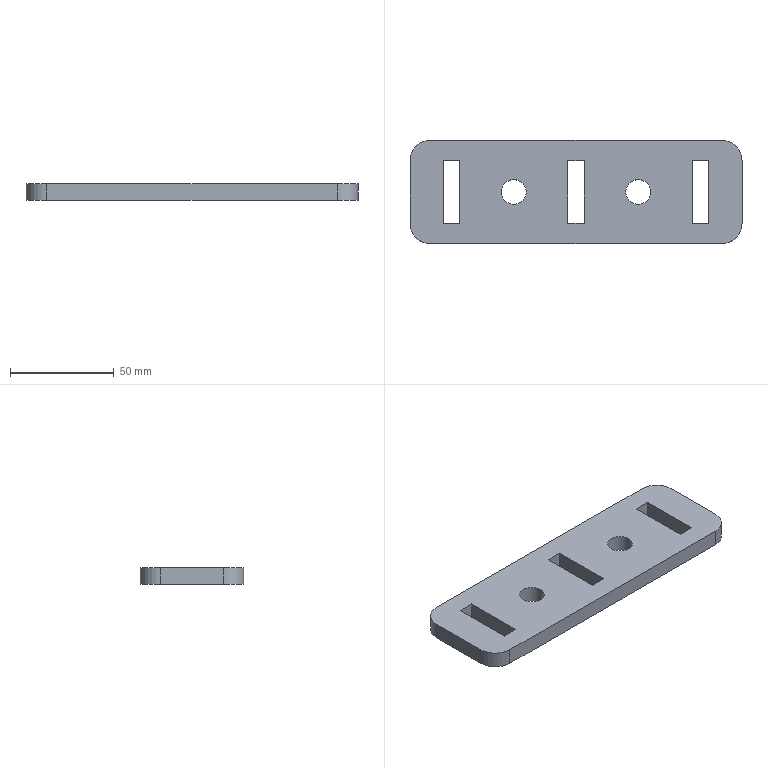Part | SolidWorks | features Fillet 1, FlatPattern 1, SMBaseFlange 1, SheetMetal 1 | 1 solid | 26 faces | box 160 x 50 x 8 mm | volume 55744 mm3 | plane 18 | cylinder 8 | commonest cylinder face diameters 12 x4 20 x4
STEP:
#1=CARTESIAN_POINT('',(-32.,480.004,8.));
#2=VERTEX_POINT('',#1);
#3=CARTESIAN_POINT('',(-20.,480.004,8.));
#4=VERTEX_POINT('',#3);
#5=CARTESIAN_POINT('',(-26.,480.004,8.));
#6=DIRECTION('',(0.,0.,1.));
#7=DIRECTION('',(1.,0.,0.));
#8=AXIS2_PLACEMENT_3D('',#5,#6,#7);
#9=CIRCLE('',#8,6.);
#10=EDGE_CURVE('',#2,#4,#9,.T.);
#11=ORIENTED_EDGE('',*,*,#10,.T.);
#12=CARTESIAN_POINT('',(-20.,480.004,0.));
#13=VERTEX_POINT('',#12);
#14=CARTESIAN_POINT('',(-20.,480.004,8.));
#15=DIRECTION('',(0.,0.,-1.));
#16=VECTOR('',#15,1000.);
#17=LINE('',#14,#16);
#18=EDGE_CURVE('',#4,#13,#17,.T.);
#19=ORIENTED_EDGE('',*,*,#18,.T.);
#20=CARTESIAN_POINT('',(-32.,480.004,0.));
#21=VERTEX_POINT('',#20);
#22=CARTESIAN_POINT('',(-26.,480.004,0.));
#23=DIRECTION('',(0.,0.,1.));
#24=DIRECTION('',(1.,0.,0.));
#25=AXIS2_PLACEMENT_3D('',#22,#23,#24);
#26=CIRCLE('',#25,6.);
#27=EDGE_CURVE('',#21,#13,#26,.T.);
#28=ORIENTED_EDGE('',*,*,#27,.F.);
#29=CARTESIAN_POINT('',(-32.,480.004,8.));
#30=DIRECTION('',(0.,0.,-1.));
#31=VECTOR('',#30,1000.);
#32=LINE('',#29,#31);
#33=EDGE_CURVE('',#2,#21,#32,.T.);
#34=ORIENTED_EDGE('',*,*,#33,.F.);
#35=EDGE_LOOP('',(#11,#19,#28,#34));
#36=FACE_OUTER_BOUND('',#35,.T.);
#37=CARTESIAN_POINT('',(-26.,480.004,8.));
#38=DIRECTION('',(0.,0.,-1.));
#39=DIRECTION('',(-1.,0.,0.));
#40=AXIS2_PLACEMENT_3D('',#37,#38,#39);
#41=CYLINDRICAL_SURFACE('',#40,6.);
#42=ADVANCED_FACE('',(#36),#41,.F.);
#43=CARTESIAN_POINT('',(28.,480.004,8.));
#44=VERTEX_POINT('',#43);
#45=CARTESIAN_POINT('',(40.,480.004,8.));
#46=VERTEX_POINT('',#45);
#47=CARTESIAN_POINT('',(34.,480.004,8.));
#48=DIRECTION('',(0.,0.,1.));
#49=DIRECTION('',(1.,0.,0.));
#50=AXIS2_PLACEMENT_3D('',#47,#48,#49);
#51=CIRCLE('',#50,6.);
#52=EDGE_CURVE('',#44,#46,#51,.T.);
#53=ORIENTED_EDGE('',*,*,#52,.T.);
#54=CARTESIAN_POINT('',(40.,480.004,0.));
#55=VERTEX_POINT('',#54);
#56=CARTESIAN_POINT('',(40.,480.004,8.));
#57=DIRECTION('',(0.,0.,-1.));
#58=VECTOR('',#57,1000.);
#59=LINE('',#56,#58);
#60=EDGE_CURVE('',#46,#55,#59,.T.);
#61=ORIENTED_EDGE('',*,*,#60,.T.);
#62=CARTESIAN_POINT('',(28.,480.004,0.));
#63=VERTEX_POINT('',#62);
#64=CARTESIAN_POINT('',(34.,480.004,0.));
#65=DIRECTION('',(0.,0.,1.));
#66=DIRECTION('',(1.,0.,0.));
#67=AXIS2_PLACEMENT_3D('',#64,#65,#66);
#68=CIRCLE('',#67,6.);
#69=EDGE_CURVE('',#63,#55,#68,.T.);
#70=ORIENTED_EDGE('',*,*,#69,.F.);
#71=CARTESIAN_POINT('',(28.,480.004,8.));
#72=DIRECTION('',(0.,0.,-1.));
#73=VECTOR('',#72,1000.);
#74=LINE('',#71,#73);
#75=EDGE_CURVE('',#44,#63,#74,.T.);
#76=ORIENTED_EDGE('',*,*,#75,.F.);
#77=EDGE_LOOP('',(#53,#61,#70,#76));
#78=FACE_OUTER_BOUND('',#77,.T.);
#79=CARTESIAN_POINT('',(34.,480.004,8.));
#80=DIRECTION('',(0.,0.,-1.));
#81=DIRECTION('',(-1.,0.,0.));
#82=AXIS2_PLACEMENT_3D('',#79,#80,#81);
#83=CYLINDRICAL_SURFACE('',#82,6.);
#84=ADVANCED_FACE('',(#78),#83,.F.);
#85=CARTESIAN_POINT('',(8.,465.004,8.));
#86=VERTEX_POINT('',#85);
#87=CARTESIAN_POINT('',(8.,495.004,8.));
#88=VERTEX_POINT('',#87);
#89=CARTESIAN_POINT('',(8.,495.004,8.));
#90=DIRECTION('',(0.,1.,0.));
#91=VECTOR('',#90,1000.);
#92=LINE('',#89,#91);
#93=EDGE_CURVE('',#86,#88,#92,.T.);
#94=ORIENTED_EDGE('',*,*,#93,.F.);
#95=CARTESIAN_POINT('',(0.,465.004,8.));
#96=VERTEX_POINT('',#95);
#97=CARTESIAN_POINT('',(8.,465.004,8.));
#98=DIRECTION('',(1.,0.,0.));
#99=VECTOR('',#98,1000.);
#100=LINE('',#97,#99);
#101=EDGE_CURVE('',#96,#86,#100,.T.);
#102=ORIENTED_EDGE('',*,*,#101,.F.);
#103=CARTESIAN_POINT('',(0.,495.004,8.));
#104=VERTEX_POINT('',#103);
#105=CARTESIAN_POINT('',(0.,495.004,8.));
#106=DIRECTION('',(0.,-1.,0.));
#107=VECTOR('',#106,1000.);
#108=LINE('',#105,#107);
#109=EDGE_CURVE('',#104,#96,#108,.T.);
#110=ORIENTED_EDGE('',*,*,#109,.F.);
#111=CARTESIAN_POINT('',(8.,495.004,8.));
#112=DIRECTION('',(-1.,0.,0.));
#113=VECTOR('',#112,1000.);
#114=LINE('',#111,#113);
#115=EDGE_CURVE('',#88,#104,#114,.T.);
#116=ORIENTED_EDGE('',*,*,#115,.F.);
#117=EDGE_LOOP('',(#94,#102,#110,#116));
#118=FACE_BOUND('',#117,.T.);
#119=CARTESIAN_POINT('',(84.,465.004,8.));
#120=VERTEX_POINT('',#119);
#121=CARTESIAN_POINT('',(84.,495.004,8.));
#122=VERTEX_POINT('',#121);
#123=CARTESIAN_POINT('',(84.,505.004,8.));
#124=DIRECTION('',(0.,1.,0.));
#125=VECTOR('',#124,1000.);
#126=LINE('',#123,#125);
#127=EDGE_CURVE('',#120,#122,#126,.T.);
#128=ORIENTED_EDGE('',*,*,#127,.T.);
#129=CARTESIAN_POINT('',(74.,505.004,8.));
#130=VERTEX_POINT('',#129);
#131=CARTESIAN_POINT('',(74.,495.004,8.));
#132=DIRECTION('',(0.,0.,1.));
#133=DIRECTION('',(-1.,0.,0.));
#134=AXIS2_PLACEMENT_3D('',#131,#132,#133);
#135=CIRCLE('',#134,10.);
#136=EDGE_CURVE('',#122,#130,#135,.T.);
#137=ORIENTED_EDGE('',*,*,#136,.T.);
#138=CARTESIAN_POINT('',(-66.,505.004,8.));
#139=VERTEX_POINT('',#138);
#140=CARTESIAN_POINT('',(84.,505.004,8.));
#141=DIRECTION('',(-1.,0.,0.));
#142=VECTOR('',#141,1000.);
#143=LINE('',#140,#142);
#144=EDGE_CURVE('',#130,#139,#143,.T.);
#145=ORIENTED_EDGE('',*,*,#144,.T.);
#146=CARTESIAN_POINT('',(-76.,495.004,8.));
#147=VERTEX_POINT('',#146);
#148=CARTESIAN_POINT('',(-66.,495.004,8.));
#149=DIRECTION('',(0.,0.,1.));
#150=DIRECTION('',(-1.,0.,0.));
#151=AXIS2_PLACEMENT_3D('',#148,#149,#150);
#152=CIRCLE('',#151,10.);
#153=EDGE_CURVE('',#139,#147,#152,.T.);
#154=ORIENTED_EDGE('',*,*,#153,.T.);
#155=CARTESIAN_POINT('',(-76.,465.004,8.));
#156=VERTEX_POINT('',#155);
#157=CARTESIAN_POINT('',(-76.,505.004,8.));
#158=DIRECTION('',(0.,-1.,0.));
#159=VECTOR('',#158,1000.);
#160=LINE('',#157,#159);
#161=EDGE_CURVE('',#147,#156,#160,.T.);
#162=ORIENTED_EDGE('',*,*,#161,.T.);
#163=CARTESIAN_POINT('',(-66.,455.004,8.));
#164=VERTEX_POINT('',#163);
#165=CARTESIAN_POINT('',(-66.,465.004,8.));
#166=DIRECTION('',(0.,0.,1.));
#167=DIRECTION('',(-1.,0.,0.));
#168=AXIS2_PLACEMENT_3D('',#165,#166,#167);
#169=CIRCLE('',#168,10.);
#170=EDGE_CURVE('',#156,#164,#169,.T.);
#171=ORIENTED_EDGE('',*,*,#170,.T.);
#172=CARTESIAN_POINT('',(74.,455.004,8.));
#173=VERTEX_POINT('',#172);
#174=CARTESIAN_POINT('',(84.,455.004,8.));
#175=DIRECTION('',(1.,0.,0.));
#176=VECTOR('',#175,1000.);
#177=LINE('',#174,#176);
#178=EDGE_CURVE('',#164,#173,#177,.T.);
#179=ORIENTED_EDGE('',*,*,#178,.T.);
#180=CARTESIAN_POINT('',(74.,465.004,8.));
#181=DIRECTION('',(0.,0.,1.));
#182=DIRECTION('',(-1.,0.,0.));
#183=AXIS2_PLACEMENT_3D('',#180,#181,#182);
#184=CIRCLE('',#183,10.);
#185=EDGE_CURVE('',#173,#120,#184,.T.);
#186=ORIENTED_EDGE('',*,*,#185,.T.);
#187=EDGE_LOOP('',(#128,#137,#145,#154,#162,#171,#179,#186));
#188=FACE_OUTER_BOUND('',#187,.T.);
#189=CARTESIAN_POINT('',(68.,465.004,8.));
#190=VERTEX_POINT('',#189);
#191=CARTESIAN_POINT('',(68.,495.004,8.));
#192=VERTEX_POINT('',#191);
#193=CARTESIAN_POINT('',(68.,495.004,8.));
#194=DIRECTION('',(0.,1.,0.));
#195=VECTOR('',#194,1000.);
#196=LINE('',#193,#195);
#197=EDGE_CURVE('',#190,#192,#196,.T.);
#198=ORIENTED_EDGE('',*,*,#197,.F.);
#199=CARTESIAN_POINT('',(60.,465.004,8.));
#200=VERTEX_POINT('',#199);
#201=CARTESIAN_POINT('',(68.,465.004,8.));
#202=DIRECTION('',(1.,0.,0.));
#203=VECTOR('',#202,1000.);
#204=LINE('',#201,#203);
#205=EDGE_CURVE('',#200,#190,#204,.T.);
#206=ORIENTED_EDGE('',*,*,#205,.F.);
#207=CARTESIAN_POINT('',(60.,495.004,8.));
#208=VERTEX_POINT('',#207);
#209=CARTESIAN_POINT('',(60.,495.004,8.));
#210=DIRECTION('',(0.,-1.,0.));
#211=VECTOR('',#210,1000.);
#212=LINE('',#209,#211);
#213=EDGE_CURVE('',#208,#200,#212,.T.);
#214=ORIENTED_EDGE('',*,*,#213,.F.);
#215=CARTESIAN_POINT('',(68.,495.004,8.));
#216=DIRECTION('',(-1.,0.,0.));
#217=VECTOR('',#216,1000.);
#218=LINE('',#215,#217);
#219=EDGE_CURVE('',#192,#208,#218,.T.);
#220=ORIENTED_EDGE('',*,*,#219,.F.);
#221=EDGE_LOOP('',(#198,#206,#214,#220));
#222=FACE_BOUND('',#221,.T.);
#223=CARTESIAN_POINT('',(-60.,495.004,8.));
#224=VERTEX_POINT('',#223);
#225=CARTESIAN_POINT('',(-60.,465.004,8.));
#226=VERTEX_POINT('',#225);
#227=CARTESIAN_POINT('',(-60.,465.004,8.));
#228=DIRECTION('',(0.,-1.,0.));
#229=VECTOR('',#228,1000.);
#230=LINE('',#227,#229);
#231=EDGE_CURVE('',#224,#226,#230,.T.);
#232=ORIENTED_EDGE('',*,*,#231,.F.);
#233=CARTESIAN_POINT('',(-52.,495.004,8.));
#234=VERTEX_POINT('',#233);
#235=CARTESIAN_POINT('',(-60.,495.004,8.));
#236=DIRECTION('',(-1.,0.,0.));
#237=VECTOR('',#236,1000.);
#238=LINE('',#235,#237);
#239=EDGE_CURVE('',#234,#224,#238,.T.);
#240=ORIENTED_EDGE('',*,*,#239,.F.);
#241=CARTESIAN_POINT('',(-52.,465.004,8.));
#242=VERTEX_POINT('',#241);
#243=CARTESIAN_POINT('',(-52.,465.004,8.));
#244=DIRECTION('',(0.,1.,0.));
#245=VECTOR('',#244,1000.);
#246=LINE('',#243,#245);
#247=EDGE_CURVE('',#242,#234,#246,.T.);
#248=ORIENTED_EDGE('',*,*,#247,.F.);
#249=CARTESIAN_POINT('',(-60.,465.004,8.));
#250=DIRECTION('',(1.,0.,0.));
#251=VECTOR('',#250,1000.);
#252=LINE('',#249,#251);
#253=EDGE_CURVE('',#226,#242,#252,.T.);
#254=ORIENTED_EDGE('',*,*,#253,.F.);
#255=EDGE_LOOP('',(#232,#240,#248,#254));
#256=FACE_BOUND('',#255,.T.);
#257=ORIENTED_EDGE('',*,*,#52,.F.);
#258=CARTESIAN_POINT('',(34.,480.004,8.));
#259=DIRECTION('',(0.,0.,1.));
#260=DIRECTION('',(1.,0.,0.));
#261=AXIS2_PLACEMENT_3D('',#258,#259,#260);
#262=CIRCLE('',#261,6.);
#263=EDGE_CURVE('',#46,#44,#262,.T.);
#264=ORIENTED_EDGE('',*,*,#263,.F.);
#265=EDGE_LOOP('',(#257,#264));
#266=FACE_BOUND('',#265,.T.);
#267=ORIENTED_EDGE('',*,*,#10,.F.);
#268=CARTESIAN_POINT('',(-26.,480.004,8.));
#269=DIRECTION('',(0.,0.,1.));
#270=DIRECTION('',(1.,0.,0.));
#271=AXIS2_PLACEMENT_3D('',#268,#269,#270);
#272=CIRCLE('',#271,6.);
#273=EDGE_CURVE('',#4,#2,#272,.T.);
#274=ORIENTED_EDGE('',*,*,#273,.F.);
#275=EDGE_LOOP('',(#267,#274));
#276=FACE_BOUND('',#275,.T.);
#277=CARTESIAN_POINT('',(0.,0.,8.));
#278=DIRECTION('',(0.,0.,-1.));
#279=DIRECTION('',(-1.,0.,0.));
#280=AXIS2_PLACEMENT_3D('',#277,#278,#279);
#281=PLANE('',#280);
#282=ADVANCED_FACE('',(#118,#188,#222,#256,#266,#276),#281,.F.);
#283=ORIENTED_EDGE('',*,*,#69,.T.);
#284=CARTESIAN_POINT('',(34.,480.004,0.));
#285=DIRECTION('',(0.,0.,1.));
#286=DIRECTION('',(1.,0.,0.));
#287=AXIS2_PLACEMENT_3D('',#284,#285,#286);
#288=CIRCLE('',#287,6.);
#289=EDGE_CURVE('',#55,#63,#288,.T.);
#290=ORIENTED_EDGE('',*,*,#289,.T.);
#291=EDGE_LOOP('',(#283,#290));
#292=FACE_BOUND('',#291,.T.);
#293=CARTESIAN_POINT('',(74.,505.004,0.));
#294=VERTEX_POINT('',#293);
#295=CARTESIAN_POINT('',(-66.,505.004,0.));
#296=VERTEX_POINT('',#295);
#297=CARTESIAN_POINT('',(84.,505.004,0.));
#298=DIRECTION('',(-1.,0.,0.));
#299=VECTOR('',#298,1000.);
#300=LINE('',#297,#299);
#301=EDGE_CURVE('',#294,#296,#300,.T.);
#302=ORIENTED_EDGE('',*,*,#301,.F.);
#303=CARTESIAN_POINT('',(84.,495.004,0.));
#304=VERTEX_POINT('',#303);
#305=CARTESIAN_POINT('',(74.,495.004,0.));
#306=DIRECTION('',(0.,0.,-1.));
#307=DIRECTION('',(-1.,0.,0.));
#308=AXIS2_PLACEMENT_3D('',#305,#306,#307);
#309=CIRCLE('',#308,10.);
#310=EDGE_CURVE('',#294,#304,#309,.T.);
#311=ORIENTED_EDGE('',*,*,#310,.T.);
#312=CARTESIAN_POINT('',(84.,465.004,0.));
#313=VERTEX_POINT('',#312);
#314=CARTESIAN_POINT('',(84.,505.004,0.));
#315=DIRECTION('',(0.,1.,0.));
#316=VECTOR('',#315,1000.);
#317=LINE('',#314,#316);
#318=EDGE_CURVE('',#313,#304,#317,.T.);
#319=ORIENTED_EDGE('',*,*,#318,.F.);
#320=CARTESIAN_POINT('',(74.,455.004,0.));
#321=VERTEX_POINT('',#320);
#322=CARTESIAN_POINT('',(74.,465.004,0.));
#323=DIRECTION('',(0.,0.,-1.));
#324=DIRECTION('',(-1.,0.,0.));
#325=AXIS2_PLACEMENT_3D('',#322,#323,#324);
#326=CIRCLE('',#325,10.);
#327=EDGE_CURVE('',#313,#321,#326,.T.);
#328=ORIENTED_EDGE('',*,*,#327,.T.);
#329=CARTESIAN_POINT('',(-66.,455.004,0.));
#330=VERTEX_POINT('',#329);
#331=CARTESIAN_POINT('',(84.,455.004,0.));
#332=DIRECTION('',(1.,0.,0.));
#333=VECTOR('',#332,1000.);
#334=LINE('',#331,#333);
#335=EDGE_CURVE('',#330,#321,#334,.T.);
#336=ORIENTED_EDGE('',*,*,#335,.F.);
#337=CARTESIAN_POINT('',(-76.,465.004,0.));
#338=VERTEX_POINT('',#337);
#339=CARTESIAN_POINT('',(-66.,465.004,0.));
#340=DIRECTION('',(0.,0.,-1.));
#341=DIRECTION('',(-1.,0.,0.));
#342=AXIS2_PLACEMENT_3D('',#339,#340,#341);
#343=CIRCLE('',#342,10.);
#344=EDGE_CURVE('',#330,#338,#343,.T.);
#345=ORIENTED_EDGE('',*,*,#344,.T.);
#346=CARTESIAN_POINT('',(-76.,495.004,0.));
#347=VERTEX_POINT('',#346);
#348=CARTESIAN_POINT('',(-76.,505.004,0.));
#349=DIRECTION('',(0.,-1.,0.));
#350=VECTOR('',#349,1000.);
#351=LINE('',#348,#350);
#352=EDGE_CURVE('',#347,#338,#351,.T.);
#353=ORIENTED_EDGE('',*,*,#352,.F.);
#354=CARTESIAN_POINT('',(-66.,495.004,0.));
#355=DIRECTION('',(0.,0.,-1.));
#356=DIRECTION('',(-1.,0.,0.));
#357=AXIS2_PLACEMENT_3D('',#354,#355,#356);
#358=CIRCLE('',#357,10.);
#359=EDGE_CURVE('',#347,#296,#358,.T.);
#360=ORIENTED_EDGE('',*,*,#359,.T.);
#361=EDGE_LOOP('',(#302,#311,#319,#328,#336,#345,#353,#360));
#362=FACE_OUTER_BOUND('',#361,.T.);
#363=CARTESIAN_POINT('',(60.,465.004,0.));
#364=VERTEX_POINT('',#363);
#365=CARTESIAN_POINT('',(68.,465.004,0.));
#366=VERTEX_POINT('',#365);
#367=CARTESIAN_POINT('',(68.,465.004,0.));
#368=DIRECTION('',(1.,0.,0.));
#369=VECTOR('',#368,1000.);
#370=LINE('',#367,#369);
#371=EDGE_CURVE('',#364,#366,#370,.T.);
#372=ORIENTED_EDGE('',*,*,#371,.T.);
#373=CARTESIAN_POINT('',(68.,495.004,0.));
#374=VERTEX_POINT('',#373);
#375=CARTESIAN_POINT('',(68.,495.004,0.));
#376=DIRECTION('',(0.,1.,0.));
#377=VECTOR('',#376,1000.);
#378=LINE('',#375,#377);
#379=EDGE_CURVE('',#366,#374,#378,.T.);
#380=ORIENTED_EDGE('',*,*,#379,.T.);
#381=CARTESIAN_POINT('',(60.,495.004,0.));
#382=VERTEX_POINT('',#381);
#383=CARTESIAN_POINT('',(68.,495.004,0.));
#384=DIRECTION('',(-1.,0.,0.));
#385=VECTOR('',#384,1000.);
#386=LINE('',#383,#385);
#387=EDGE_CURVE('',#374,#382,#386,.T.);
#388=ORIENTED_EDGE('',*,*,#387,.T.);
#389=CARTESIAN_POINT('',(60.,495.004,0.));
#390=DIRECTION('',(0.,-1.,0.));
#391=VECTOR('',#390,1000.);
#392=LINE('',#389,#391);
#393=EDGE_CURVE('',#382,#364,#392,.T.);
#394=ORIENTED_EDGE('',*,*,#393,.T.);
#395=EDGE_LOOP('',(#372,#380,#388,#394));
#396=FACE_BOUND('',#395,.T.);
#397=CARTESIAN_POINT('',(0.,465.004,0.));
#398=VERTEX_POINT('',#397);
#399=CARTESIAN_POINT('',(8.,465.004,0.));
#400=VERTEX_POINT('',#399);
#401=CARTESIAN_POINT('',(8.,465.004,0.));
#402=DIRECTION('',(1.,0.,0.));
#403=VECTOR('',#402,1000.);
#404=LINE('',#401,#403);
#405=EDGE_CURVE('',#398,#400,#404,.T.);
#406=ORIENTED_EDGE('',*,*,#405,.T.);
#407=CARTESIAN_POINT('',(8.,495.004,0.));
#408=VERTEX_POINT('',#407);
#409=CARTESIAN_POINT('',(8.,495.004,0.));
#410=DIRECTION('',(0.,1.,0.));
#411=VECTOR('',#410,1000.);
#412=LINE('',#409,#411);
#413=EDGE_CURVE('',#400,#408,#412,.T.);
#414=ORIENTED_EDGE('',*,*,#413,.T.);
#415=CARTESIAN_POINT('',(0.,495.004,0.));
#416=VERTEX_POINT('',#415);
#417=CARTESIAN_POINT('',(8.,495.004,0.));
#418=DIRECTION('',(-1.,0.,0.));
#419=VECTOR('',#418,1000.);
#420=LINE('',#417,#419);
#421=EDGE_CURVE('',#408,#416,#420,.T.);
#422=ORIENTED_EDGE('',*,*,#421,.T.);
#423=CARTESIAN_POINT('',(0.,495.004,0.));
#424=DIRECTION('',(0.,-1.,0.));
#425=VECTOR('',#424,1000.);
#426=LINE('',#423,#425);
#427=EDGE_CURVE('',#416,#398,#426,.T.);
#428=ORIENTED_EDGE('',*,*,#427,.T.);
#429=EDGE_LOOP('',(#406,#414,#422,#428));
#430=FACE_BOUND('',#429,.T.);
#431=CARTESIAN_POINT('',(-52.,495.004,0.));
#432=VERTEX_POINT('',#431);
#433=CARTESIAN_POINT('',(-60.,495.004,0.));
#434=VERTEX_POINT('',#433);
#435=CARTESIAN_POINT('',(-60.,495.004,0.));
#436=DIRECTION('',(-1.,0.,0.));
#437=VECTOR('',#436,1000.);
#438=LINE('',#435,#437);
#439=EDGE_CURVE('',#432,#434,#438,.T.);
#440=ORIENTED_EDGE('',*,*,#439,.T.);
#441=CARTESIAN_POINT('',(-60.,465.004,0.));
#442=VERTEX_POINT('',#441);
#443=CARTESIAN_POINT('',(-60.,465.004,0.));
#444=DIRECTION('',(0.,-1.,0.));
#445=VECTOR('',#444,1000.);
#446=LINE('',#443,#445);
#447=EDGE_CURVE('',#434,#442,#446,.T.);
#448=ORIENTED_EDGE('',*,*,#447,.T.);
#449=CARTESIAN_POINT('',(-52.,465.004,0.));
#450=VERTEX_POINT('',#449);
#451=CARTESIAN_POINT('',(-60.,465.004,0.));
#452=DIRECTION('',(1.,0.,0.));
#453=VECTOR('',#452,1000.);
#454=LINE('',#451,#453);
#455=EDGE_CURVE('',#442,#450,#454,.T.);
#456=ORIENTED_EDGE('',*,*,#455,.T.);
#457=CARTESIAN_POINT('',(-52.,465.004,0.));
#458=DIRECTION('',(0.,1.,0.));
#459=VECTOR('',#458,1000.);
#460=LINE('',#457,#459);
#461=EDGE_CURVE('',#450,#432,#460,.T.);
#462=ORIENTED_EDGE('',*,*,#461,.T.);
#463=EDGE_LOOP('',(#440,#448,#456,#462));
#464=FACE_BOUND('',#463,.T.);
#465=ORIENTED_EDGE('',*,*,#27,.T.);
#466=CARTESIAN_POINT('',(-26.,480.004,0.));
#467=DIRECTION('',(0.,0.,1.));
#468=DIRECTION('',(1.,0.,0.));
#469=AXIS2_PLACEMENT_3D('',#466,#467,#468);
#470=CIRCLE('',#469,6.);
#471=EDGE_CURVE('',#13,#21,#470,.T.);
#472=ORIENTED_EDGE('',*,*,#471,.T.);
#473=EDGE_LOOP('',(#465,#472));
#474=FACE_BOUND('',#473,.T.);
#475=CARTESIAN_POINT('',(0.,0.,0.));
#476=DIRECTION('',(0.,0.,-1.));
#477=DIRECTION('',(-1.,0.,0.));
#478=AXIS2_PLACEMENT_3D('',#475,#476,#477);
#479=PLANE('',#478);
#480=ADVANCED_FACE('',(#292,#362,#396,#430,#464,#474),#479,.T.);
#481=ORIENTED_EDGE('',*,*,#318,.T.);
#482=CARTESIAN_POINT('',(84.,495.004,8.));
#483=DIRECTION('',(0.,0.,1.));
#484=VECTOR('',#483,1000.);
#485=LINE('',#482,#484);
#486=EDGE_CURVE('',#304,#122,#485,.T.);
#487=ORIENTED_EDGE('',*,*,#486,.T.);
#488=ORIENTED_EDGE('',*,*,#127,.F.);
#489=CARTESIAN_POINT('',(84.,465.004,8.));
#490=DIRECTION('',(0.,0.,-1.));
#491=VECTOR('',#490,1000.);
#492=LINE('',#489,#491);
#493=EDGE_CURVE('',#120,#313,#492,.T.);
#494=ORIENTED_EDGE('',*,*,#493,.T.);
#495=EDGE_LOOP('',(#481,#487,#488,#494));
#496=FACE_OUTER_BOUND('',#495,.T.);
#497=CARTESIAN_POINT('',(84.,505.004,8.));
#498=DIRECTION('',(-1.,0.,0.));
#499=DIRECTION('',(0.,0.,1.));
#500=AXIS2_PLACEMENT_3D('',#497,#498,#499);
#501=PLANE('',#500);
#502=ADVANCED_FACE('',(#496),#501,.F.);
#503=ORIENTED_EDGE('',*,*,#144,.F.);
#504=CARTESIAN_POINT('',(74.,505.004,8.));
#505=DIRECTION('',(0.,0.,-1.));
#506=VECTOR('',#505,1000.);
#507=LINE('',#504,#506);
#508=EDGE_CURVE('',#130,#294,#507,.T.);
#509=ORIENTED_EDGE('',*,*,#508,.T.);
#510=ORIENTED_EDGE('',*,*,#301,.T.);
#511=CARTESIAN_POINT('',(-66.,505.004,8.));
#512=DIRECTION('',(0.,0.,1.));
#513=VECTOR('',#512,1000.);
#514=LINE('',#511,#513);
#515=EDGE_CURVE('',#296,#139,#514,.T.);
#516=ORIENTED_EDGE('',*,*,#515,.T.);
#517=EDGE_LOOP('',(#503,#509,#510,#516));
#518=FACE_OUTER_BOUND('',#517,.T.);
#519=CARTESIAN_POINT('',(84.,505.004,8.));
#520=DIRECTION('',(0.,-1.,0.));
#521=DIRECTION('',(0.,0.,-1.));
#522=AXIS2_PLACEMENT_3D('',#519,#520,#521);
#523=PLANE('',#522);
#524=ADVANCED_FACE('',(#518),#523,.F.);
#525=ORIENTED_EDGE('',*,*,#161,.F.);
#526=CARTESIAN_POINT('',(-76.,495.004,8.));
#527=DIRECTION('',(0.,0.,-1.));
#528=VECTOR('',#527,1000.);
#529=LINE('',#526,#528);
#530=EDGE_CURVE('',#147,#347,#529,.T.);
#531=ORIENTED_EDGE('',*,*,#530,.T.);
#532=ORIENTED_EDGE('',*,*,#352,.T.);
#533=CARTESIAN_POINT('',(-76.,465.004,8.));
#534=DIRECTION('',(0.,0.,1.));
#535=VECTOR('',#534,1000.);
#536=LINE('',#533,#535);
#537=EDGE_CURVE('',#338,#156,#536,.T.);
#538=ORIENTED_EDGE('',*,*,#537,.T.);
#539=EDGE_LOOP('',(#525,#531,#532,#538));
#540=FACE_OUTER_BOUND('',#539,.T.);
#541=CARTESIAN_POINT('',(-76.,505.004,8.));
#542=DIRECTION('',(1.,0.,0.));
#543=DIRECTION('',(0.,0.,-1.));
#544=AXIS2_PLACEMENT_3D('',#541,#542,#543);
#545=PLANE('',#544);
#546=ADVANCED_FACE('',(#540),#545,.F.);
#547=ORIENTED_EDGE('',*,*,#335,.T.);
#548=CARTESIAN_POINT('',(74.,455.004,8.));
#549=DIRECTION('',(0.,0.,1.));
#550=VECTOR('',#549,1000.);
#551=LINE('',#548,#550);
#552=EDGE_CURVE('',#321,#173,#551,.T.);
#553=ORIENTED_EDGE('',*,*,#552,.T.);
#554=ORIENTED_EDGE('',*,*,#178,.F.);
#555=CARTESIAN_POINT('',(-66.,455.004,8.));
#556=DIRECTION('',(0.,0.,-1.));
#557=VECTOR('',#556,1000.);
#558=LINE('',#555,#557);
#559=EDGE_CURVE('',#164,#330,#558,.T.);
#560=ORIENTED_EDGE('',*,*,#559,.T.);
#561=EDGE_LOOP('',(#547,#553,#554,#560));
#562=FACE_OUTER_BOUND('',#561,.T.);
#563=CARTESIAN_POINT('',(84.,455.004,8.));
#564=DIRECTION('',(0.,1.,0.));
#565=DIRECTION('',(0.,0.,1.));
#566=AXIS2_PLACEMENT_3D('',#563,#564,#565);
#567=PLANE('',#566);
#568=ADVANCED_FACE('',(#562),#567,.F.);
#569=ORIENTED_EDGE('',*,*,#379,.F.);
#570=CARTESIAN_POINT('',(68.,465.004,8.));
#571=DIRECTION('',(0.,0.,-1.));
#572=VECTOR('',#571,1000.);
#573=LINE('',#570,#572);
#574=EDGE_CURVE('',#190,#366,#573,.T.);
#575=ORIENTED_EDGE('',*,*,#574,.F.);
#576=ORIENTED_EDGE('',*,*,#197,.T.);
#577=CARTESIAN_POINT('',(68.,495.004,8.));
#578=DIRECTION('',(0.,0.,-1.));
#579=VECTOR('',#578,1000.);
#580=LINE('',#577,#579);
#581=EDGE_CURVE('',#192,#374,#580,.T.);
#582=ORIENTED_EDGE('',*,*,#581,.T.);
#583=EDGE_LOOP('',(#569,#575,#576,#582));
#584=FACE_OUTER_BOUND('',#583,.T.);
#585=CARTESIAN_POINT('',(68.,495.004,8.));
#586=DIRECTION('',(-1.,0.,0.));
#587=DIRECTION('',(0.,0.,1.));
#588=AXIS2_PLACEMENT_3D('',#585,#586,#587);
#589=PLANE('',#588);
#590=ADVANCED_FACE('',(#584),#589,.T.);
#591=ORIENTED_EDGE('',*,*,#387,.F.);
#592=ORIENTED_EDGE('',*,*,#581,.F.);
#593=ORIENTED_EDGE('',*,*,#219,.T.);
#594=CARTESIAN_POINT('',(60.,495.004,8.));
#595=DIRECTION('',(0.,0.,-1.));
#596=VECTOR('',#595,1000.);
#597=LINE('',#594,#596);
#598=EDGE_CURVE('',#208,#382,#597,.T.);
#599=ORIENTED_EDGE('',*,*,#598,.T.);
#600=EDGE_LOOP('',(#591,#592,#593,#599));
#601=FACE_OUTER_BOUND('',#600,.T.);
#602=CARTESIAN_POINT('',(68.,495.004,8.));
#603=DIRECTION('',(0.,-1.,0.));
#604=DIRECTION('',(0.,0.,-1.));
#605=AXIS2_PLACEMENT_3D('',#602,#603,#604);
#606=PLANE('',#605);
#607=ADVANCED_FACE('',(#601),#606,.T.);
#608=ORIENTED_EDGE('',*,*,#393,.F.);
#609=ORIENTED_EDGE('',*,*,#598,.F.);
#610=ORIENTED_EDGE('',*,*,#213,.T.);
#611=CARTESIAN_POINT('',(60.,465.004,8.));
#612=DIRECTION('',(0.,0.,-1.));
#613=VECTOR('',#612,1000.);
#614=LINE('',#611,#613);
#615=EDGE_CURVE('',#200,#364,#614,.T.);
#616=ORIENTED_EDGE('',*,*,#615,.T.);
#617=EDGE_LOOP('',(#608,#609,#610,#616));
#618=FACE_OUTER_BOUND('',#617,.T.);
#619=CARTESIAN_POINT('',(60.,495.004,8.));
#620=DIRECTION('',(1.,0.,0.));
#621=DIRECTION('',(0.,0.,-1.));
#622=AXIS2_PLACEMENT_3D('',#619,#620,#621);
#623=PLANE('',#622);
#624=ADVANCED_FACE('',(#618),#623,.T.);
#625=ORIENTED_EDGE('',*,*,#371,.F.);
#626=ORIENTED_EDGE('',*,*,#615,.F.);
#627=ORIENTED_EDGE('',*,*,#205,.T.);
#628=ORIENTED_EDGE('',*,*,#574,.T.);
#629=EDGE_LOOP('',(#625,#626,#627,#628));
#630=FACE_OUTER_BOUND('',#629,.T.);
#631=CARTESIAN_POINT('',(68.,465.004,8.));
#632=DIRECTION('',(0.,1.,0.));
#633=DIRECTION('',(0.,0.,1.));
#634=AXIS2_PLACEMENT_3D('',#631,#632,#633);
#635=PLANE('',#634);
#636=ADVANCED_FACE('',(#630),#635,.T.);
#637=ORIENTED_EDGE('',*,*,#413,.F.);
#638=CARTESIAN_POINT('',(8.,465.004,8.));
#639=DIRECTION('',(0.,0.,-1.));
#640=VECTOR('',#639,1000.);
#641=LINE('',#638,#640);
#642=EDGE_CURVE('',#86,#400,#641,.T.);
#643=ORIENTED_EDGE('',*,*,#642,.F.);
#644=ORIENTED_EDGE('',*,*,#93,.T.);
#645=CARTESIAN_POINT('',(8.,495.004,8.));
#646=DIRECTION('',(0.,0.,-1.));
#647=VECTOR('',#646,1000.);
#648=LINE('',#645,#647);
#649=EDGE_CURVE('',#88,#408,#648,.T.);
#650=ORIENTED_EDGE('',*,*,#649,.T.);
#651=EDGE_LOOP('',(#637,#643,#644,#650));
#652=FACE_OUTER_BOUND('',#651,.T.);
#653=CARTESIAN_POINT('',(8.,495.004,8.));
#654=DIRECTION('',(-1.,0.,0.));
#655=DIRECTION('',(0.,0.,1.));
#656=AXIS2_PLACEMENT_3D('',#653,#654,#655);
#657=PLANE('',#656);
#658=ADVANCED_FACE('',(#652),#657,.T.);
#659=ORIENTED_EDGE('',*,*,#421,.F.);
#660=ORIENTED_EDGE('',*,*,#649,.F.);
#661=ORIENTED_EDGE('',*,*,#115,.T.);
#662=CARTESIAN_POINT('',(0.,495.004,8.));
#663=DIRECTION('',(0.,0.,-1.));
#664=VECTOR('',#663,1000.);
#665=LINE('',#662,#664);
#666=EDGE_CURVE('',#104,#416,#665,.T.);
#667=ORIENTED_EDGE('',*,*,#666,.T.);
#668=EDGE_LOOP('',(#659,#660,#661,#667));
#669=FACE_OUTER_BOUND('',#668,.T.);
#670=CARTESIAN_POINT('',(8.,495.004,8.));
#671=DIRECTION('',(0.,-1.,0.));
#672=DIRECTION('',(0.,0.,-1.));
#673=AXIS2_PLACEMENT_3D('',#670,#671,#672);
#674=PLANE('',#673);
#675=ADVANCED_FACE('',(#669),#674,.T.);
#676=ORIENTED_EDGE('',*,*,#427,.F.);
#677=ORIENTED_EDGE('',*,*,#666,.F.);
#678=ORIENTED_EDGE('',*,*,#109,.T.);
#679=CARTESIAN_POINT('',(0.,465.004,8.));
#680=DIRECTION('',(0.,0.,-1.));
#681=VECTOR('',#680,1000.);
#682=LINE('',#679,#681);
#683=EDGE_CURVE('',#96,#398,#682,.T.);
#684=ORIENTED_EDGE('',*,*,#683,.T.);
#685=EDGE_LOOP('',(#676,#677,#678,#684));
#686=FACE_OUTER_BOUND('',#685,.T.);
#687=CARTESIAN_POINT('',(0.,495.004,8.));
#688=DIRECTION('',(1.,0.,0.));
#689=DIRECTION('',(0.,0.,-1.));
#690=AXIS2_PLACEMENT_3D('',#687,#688,#689);
#691=PLANE('',#690);
#692=ADVANCED_FACE('',(#686),#691,.T.);
#693=ORIENTED_EDGE('',*,*,#405,.F.);
#694=ORIENTED_EDGE('',*,*,#683,.F.);
#695=ORIENTED_EDGE('',*,*,#101,.T.);
#696=ORIENTED_EDGE('',*,*,#642,.T.);
#697=EDGE_LOOP('',(#693,#694,#695,#696));
#698=FACE_OUTER_BOUND('',#697,.T.);
#699=CARTESIAN_POINT('',(8.,465.004,8.));
#700=DIRECTION('',(0.,1.,0.));
#701=DIRECTION('',(0.,0.,1.));
#702=AXIS2_PLACEMENT_3D('',#699,#700,#701);
#703=PLANE('',#702);
#704=ADVANCED_FACE('',(#698),#703,.T.);
#705=ORIENTED_EDGE('',*,*,#447,.F.);
#706=CARTESIAN_POINT('',(-60.,495.004,8.));
#707=DIRECTION('',(0.,0.,-1.));
#708=VECTOR('',#707,1000.);
#709=LINE('',#706,#708);
#710=EDGE_CURVE('',#224,#434,#709,.T.);
#711=ORIENTED_EDGE('',*,*,#710,.F.);
#712=ORIENTED_EDGE('',*,*,#231,.T.);
#713=CARTESIAN_POINT('',(-60.,465.004,8.));
#714=DIRECTION('',(0.,0.,-1.));
#715=VECTOR('',#714,1000.);
#716=LINE('',#713,#715);
#717=EDGE_CURVE('',#226,#442,#716,.T.);
#718=ORIENTED_EDGE('',*,*,#717,.T.);
#719=EDGE_LOOP('',(#705,#711,#712,#718));
#720=FACE_OUTER_BOUND('',#719,.T.);
#721=CARTESIAN_POINT('',(-60.,465.004,8.));
#722=DIRECTION('',(1.,0.,0.));
#723=DIRECTION('',(0.,0.,-1.));
#724=AXIS2_PLACEMENT_3D('',#721,#722,#723);
#725=PLANE('',#724);
#726=ADVANCED_FACE('',(#720),#725,.T.);
#727=ORIENTED_EDGE('',*,*,#455,.F.);
#728=ORIENTED_EDGE('',*,*,#717,.F.);
#729=ORIENTED_EDGE('',*,*,#253,.T.);
#730=CARTESIAN_POINT('',(-52.,465.004,8.));
#731=DIRECTION('',(0.,0.,-1.));
#732=VECTOR('',#731,1000.);
#733=LINE('',#730,#732);
#734=EDGE_CURVE('',#242,#450,#733,.T.);
#735=ORIENTED_EDGE('',*,*,#734,.T.);
#736=EDGE_LOOP('',(#727,#728,#729,#735));
#737=FACE_OUTER_BOUND('',#736,.T.);
#738=CARTESIAN_POINT('',(-60.,465.004,8.));
#739=DIRECTION('',(0.,1.,0.));
#740=DIRECTION('',(0.,0.,1.));
#741=AXIS2_PLACEMENT_3D('',#738,#739,#740);
#742=PLANE('',#741);
#743=ADVANCED_FACE('',(#737),#742,.T.);
#744=ORIENTED_EDGE('',*,*,#461,.F.);
#745=ORIENTED_EDGE('',*,*,#734,.F.);
#746=ORIENTED_EDGE('',*,*,#247,.T.);
#747=CARTESIAN_POINT('',(-52.,495.004,8.));
#748=DIRECTION('',(0.,0.,-1.));
#749=VECTOR('',#748,1000.);
#750=LINE('',#747,#749);
#751=EDGE_CURVE('',#234,#432,#750,.T.);
#752=ORIENTED_EDGE('',*,*,#751,.T.);
#753=EDGE_LOOP('',(#744,#745,#746,#752));
#754=FACE_OUTER_BOUND('',#753,.T.);
#755=CARTESIAN_POINT('',(-52.,465.004,8.));
#756=DIRECTION('',(-1.,0.,0.));
#757=DIRECTION('',(0.,0.,1.));
#758=AXIS2_PLACEMENT_3D('',#755,#756,#757);
#759=PLANE('',#758);
#760=ADVANCED_FACE('',(#754),#759,.T.);
#761=ORIENTED_EDGE('',*,*,#439,.F.);
#762=ORIENTED_EDGE('',*,*,#751,.F.);
#763=ORIENTED_EDGE('',*,*,#239,.T.);
#764=ORIENTED_EDGE('',*,*,#710,.T.);
#765=EDGE_LOOP('',(#761,#762,#763,#764));
#766=FACE_OUTER_BOUND('',#765,.T.);
#767=CARTESIAN_POINT('',(-60.,495.004,8.));
#768=DIRECTION('',(0.,-1.,0.));
#769=DIRECTION('',(0.,0.,-1.));
#770=AXIS2_PLACEMENT_3D('',#767,#768,#769);
#771=PLANE('',#770);
#772=ADVANCED_FACE('',(#766),#771,.T.);
#773=ORIENTED_EDGE('',*,*,#60,.F.);
#774=ORIENTED_EDGE('',*,*,#263,.T.);
#775=ORIENTED_EDGE('',*,*,#75,.T.);
#776=ORIENTED_EDGE('',*,*,#289,.F.);
#777=EDGE_LOOP('',(#773,#774,#775,#776));
#778=FACE_OUTER_BOUND('',#777,.T.);
#779=CARTESIAN_POINT('',(34.,480.004,8.));
#780=DIRECTION('',(0.,0.,-1.));
#781=DIRECTION('',(-1.,0.,0.));
#782=AXIS2_PLACEMENT_3D('',#779,#780,#781);
#783=CYLINDRICAL_SURFACE('',#782,6.);
#784=ADVANCED_FACE('',(#778),#783,.F.);
#785=ORIENTED_EDGE('',*,*,#18,.F.);
#786=ORIENTED_EDGE('',*,*,#273,.T.);
#787=ORIENTED_EDGE('',*,*,#33,.T.);
#788=ORIENTED_EDGE('',*,*,#471,.F.);
#789=EDGE_LOOP('',(#785,#786,#787,#788));
#790=FACE_OUTER_BOUND('',#789,.T.);
#791=CARTESIAN_POINT('',(-26.,480.004,8.));
#792=DIRECTION('',(0.,0.,-1.));
#793=DIRECTION('',(-1.,0.,0.));
#794=AXIS2_PLACEMENT_3D('',#791,#792,#793);
#795=CYLINDRICAL_SURFACE('',#794,6.);
#796=ADVANCED_FACE('',(#790),#795,.F.);
#797=ORIENTED_EDGE('',*,*,#136,.F.);
#798=ORIENTED_EDGE('',*,*,#486,.F.);
#799=ORIENTED_EDGE('',*,*,#310,.F.);
#800=ORIENTED_EDGE('',*,*,#508,.F.);
#801=EDGE_LOOP('',(#797,#798,#799,#800));
#802=FACE_OUTER_BOUND('',#801,.T.);
#803=CARTESIAN_POINT('',(74.,495.004,8.));
#804=DIRECTION('',(0.,0.,-1.));
#805=DIRECTION('',(-1.,0.,0.));
#806=AXIS2_PLACEMENT_3D('',#803,#804,#805);
#807=CYLINDRICAL_SURFACE('',#806,10.);
#808=ADVANCED_FACE('',(#802),#807,.T.);
#809=ORIENTED_EDGE('',*,*,#185,.F.);
#810=ORIENTED_EDGE('',*,*,#552,.F.);
#811=ORIENTED_EDGE('',*,*,#327,.F.);
#812=ORIENTED_EDGE('',*,*,#493,.F.);
#813=EDGE_LOOP('',(#809,#810,#811,#812));
#814=FACE_OUTER_BOUND('',#813,.T.);
#815=CARTESIAN_POINT('',(74.,465.004,8.));
#816=DIRECTION('',(0.,0.,-1.));
#817=DIRECTION('',(-1.,0.,0.));
#818=AXIS2_PLACEMENT_3D('',#815,#816,#817);
#819=CYLINDRICAL_SURFACE('',#818,10.);
#820=ADVANCED_FACE('',(#814),#819,.T.);
#821=ORIENTED_EDGE('',*,*,#153,.F.);
#822=ORIENTED_EDGE('',*,*,#515,.F.);
#823=ORIENTED_EDGE('',*,*,#359,.F.);
#824=ORIENTED_EDGE('',*,*,#530,.F.);
#825=EDGE_LOOP('',(#821,#822,#823,#824));
#826=FACE_OUTER_BOUND('',#825,.T.);
#827=CARTESIAN_POINT('',(-66.,495.004,8.));
#828=DIRECTION('',(0.,0.,-1.));
#829=DIRECTION('',(-1.,0.,0.));
#830=AXIS2_PLACEMENT_3D('',#827,#828,#829);
#831=CYLINDRICAL_SURFACE('',#830,10.);
#832=ADVANCED_FACE('',(#826),#831,.T.);
#833=ORIENTED_EDGE('',*,*,#170,.F.);
#834=ORIENTED_EDGE('',*,*,#537,.F.);
#835=ORIENTED_EDGE('',*,*,#344,.F.);
#836=ORIENTED_EDGE('',*,*,#559,.F.);
#837=EDGE_LOOP('',(#833,#834,#835,#836));
#838=FACE_OUTER_BOUND('',#837,.T.);
#839=CARTESIAN_POINT('',(-66.,465.004,8.));
#840=DIRECTION('',(0.,0.,-1.));
#841=DIRECTION('',(-1.,0.,0.));
#842=AXIS2_PLACEMENT_3D('',#839,#840,#841);
#843=CYLINDRICAL_SURFACE('',#842,10.);
#844=ADVANCED_FACE('',(#838),#843,.T.);
#845=CLOSED_SHELL('',(#42,#84,#282,#480,#502,#524,#546,#568,#590,#607,#624,#636,#658,#675,#692,#704,#726,#743,#760,#772,#784,#796,#808,#820,#832,#844));
#846=MANIFOLD_SOLID_BREP('',#845);
#847=CARTESIAN_POINT('',(0.,0.,0.));
#848=DIRECTION('',(0.,0.,1.));
#849=DIRECTION('',(1.,0.,0.));
#850=AXIS2_PLACEMENT_3D('',#847,#848,#849);
#851=(LENGTH_UNIT()NAMED_UNIT(*)SI_UNIT(.MILLI.,.METRE.));
#852=UNCERTAINTY_MEASURE_WITH_UNIT(LENGTH_MEASURE(0.00001),#851,'','');
#853=(NAMED_UNIT(*)PLANE_ANGLE_UNIT()SI_UNIT($,.RADIAN.));
#854=(NAMED_UNIT(*)SI_UNIT($,.STERADIAN.)SOLID_ANGLE_UNIT());
#855=(GEOMETRIC_REPRESENTATION_CONTEXT(3)GLOBAL_UNCERTAINTY_ASSIGNED_CONTEXT((#852))GLOBAL_UNIT_ASSIGNED_CONTEXT((#851,#853,#854))REPRESENTATION_CONTEXT('',''));
#856=ADVANCED_BREP_SHAPE_REPRESENTATION('',(#846,#850),#855);